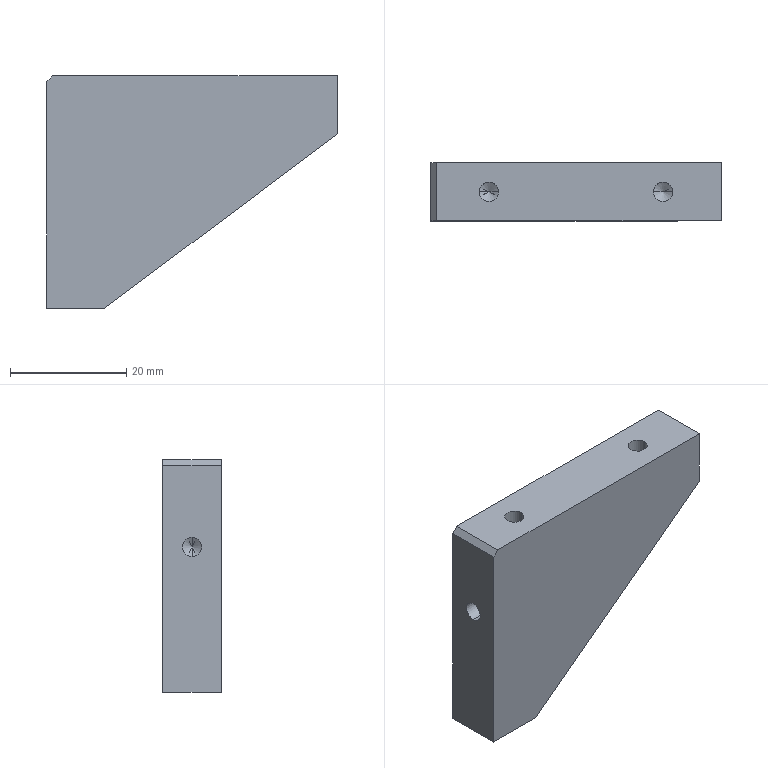Part | STEP file | PN_0035 | 1 solid | 20 faces | box 50 x 10 x 40 mm | volume 13691 mm3 | plane 8 | cylinder 6 | cone 6 | commonest cylinder face diameters 3.3 x6
STEP:
#1=CARTESIAN_POINT('',(0.,0.,0.));
#2=DIRECTION('',(0.,0.,1.));
#3=DIRECTION('',(1.,0.,0.));
#4=AXIS2_PLACEMENT_3D('',#1,#2,#3);
#5=CARTESIAN_POINT('',(16.65,5.,8.5));
#6=VERTEX_POINT('',#5);
#7=CARTESIAN_POINT('',(16.65,5.,20.));
#8=VERTEX_POINT('',#7);
#9=CARTESIAN_POINT('',(16.65,5.,20.));
#10=DIRECTION('',(0.,0.,1.));
#11=VECTOR('',#10,1.);
#12=LINE('',#9,#11);
#13=CARTESIAN_POINT('',(15.,5.,20.));
#14=DIRECTION('',(0.,0.,1.));
#15=DIRECTION('',(1.,0.,0.));
#16=AXIS2_PLACEMENT_3D('',#13,#14,#15);
#17=CYLINDRICAL_SURFACE('',#16,1.65);
#18=CARTESIAN_POINT('',(6.283,0.));
#19=DIRECTION('',(0.,1.));
#20=VECTOR('',#19,1.);
#21=LINE('',#18,#20);
#22=(GEOMETRIC_REPRESENTATION_CONTEXT(2)PARAMETRIC_REPRESENTATION_CONTEXT()REPRESENTATION_CONTEXT('',''));
#23=DEFINITIONAL_REPRESENTATION('',(#21),#22);
#24=PCURVE('',#17,#23);
#25=CARTESIAN_POINT('',(15.,5.,20.));
#26=DIRECTION('',(0.,0.,1.));
#27=DIRECTION('',(1.,0.,0.));
#28=AXIS2_PLACEMENT_3D('',#25,#26,#27);
#29=CYLINDRICAL_SURFACE('',#28,1.65);
#30=CARTESIAN_POINT('',(0.,0.));
#31=DIRECTION('',(0.,1.));
#32=VECTOR('',#31,1.);
#33=LINE('',#30,#32);
#34=(GEOMETRIC_REPRESENTATION_CONTEXT(2)PARAMETRIC_REPRESENTATION_CONTEXT()REPRESENTATION_CONTEXT('',''));
#35=DEFINITIONAL_REPRESENTATION('',(#33),#34);
#36=PCURVE('',#29,#35);
#37=SURFACE_CURVE('',#12,(#24,#36),.PCURVE_S1.);
#38=EDGE_CURVE('',#6,#8,#37,.T.);
#39=ORIENTED_EDGE('',*,*,#38,.T.);
#40=CARTESIAN_POINT('',(13.35,5.,20.));
#41=VERTEX_POINT('',#40);
#42=CARTESIAN_POINT('',(15.,5.,20.));
#43=DIRECTION('',(0.,0.,1.));
#44=DIRECTION('',(1.,0.,0.));
#45=AXIS2_PLACEMENT_3D('',#42,#43,#44);
#46=CIRCLE('',#45,1.65);
#47=CARTESIAN_POINT('',(0.,0.));
#48=DIRECTION('',(1.,0.));
#49=VECTOR('',#48,1.);
#50=LINE('',#47,#49);
#51=(GEOMETRIC_REPRESENTATION_CONTEXT(2)PARAMETRIC_REPRESENTATION_CONTEXT()REPRESENTATION_CONTEXT('',''));
#52=DEFINITIONAL_REPRESENTATION('',(#50),#51);
#53=PCURVE('',#17,#52);
#54=CARTESIAN_POINT('',(-25.,10.,20.));
#55=DIRECTION('',(0.,0.,-1.));
#56=DIRECTION('',(-1.,0.,0.));
#57=AXIS2_PLACEMENT_3D('',#54,#55,#56);
#58=PLANE('',#57);
#59=CARTESIAN_POINT('',(-41.65,-5.));
#60=CARTESIAN_POINT('',(-41.65,-2.142));
#61=CARTESIAN_POINT('',(-39.175,-3.571));
#62=CARTESIAN_POINT('',(-36.7,-5.));
#63=CARTESIAN_POINT('',(-39.175,-6.429));
#64=CARTESIAN_POINT('',(-41.65,-7.858));
#65=CARTESIAN_POINT('',(-41.65,-5.));
#66=(BOUNDED_CURVE()B_SPLINE_CURVE(2,(#59,#60,#61,#62,#63,#64,#65),.UNSPECIFIED.,.T.,.F.)B_SPLINE_CURVE_WITH_KNOTS((1,2,2,2,2,1),(-2.094,0.,2.094,4.189,6.283,8.378),.UNSPECIFIED.)CURVE()GEOMETRIC_REPRESENTATION_ITEM()RATIONAL_B_SPLINE_CURVE((1.,0.5,1.,0.5,1.,0.5,1.))REPRESENTATION_ITEM(''));
#67=(GEOMETRIC_REPRESENTATION_CONTEXT(2)PARAMETRIC_REPRESENTATION_CONTEXT()REPRESENTATION_CONTEXT('',''));
#68=DEFINITIONAL_REPRESENTATION('',(#66),#67);
#69=PCURVE('',#58,#68);
#70=SURFACE_CURVE('',#46,(#53,#69),.PCURVE_S1.);
#71=EDGE_CURVE('',#41,#8,#70,.T.);
#72=ORIENTED_EDGE('',*,*,#71,.F.);
#73=CARTESIAN_POINT('',(13.35,5.,8.5));
#74=VERTEX_POINT('',#73);
#75=CARTESIAN_POINT('',(13.35,5.,20.));
#76=DIRECTION('',(0.,0.,1.));
#77=VECTOR('',#76,1.);
#78=LINE('',#75,#77);
#79=CARTESIAN_POINT('',(3.142,0.));
#80=DIRECTION('',(0.,1.));
#81=VECTOR('',#80,1.);
#82=LINE('',#79,#81);
#83=(GEOMETRIC_REPRESENTATION_CONTEXT(2)PARAMETRIC_REPRESENTATION_CONTEXT()REPRESENTATION_CONTEXT('',''));
#84=DEFINITIONAL_REPRESENTATION('',(#82),#83);
#85=PCURVE('',#17,#84);
#86=CARTESIAN_POINT('',(3.142,0.));
#87=DIRECTION('',(0.,1.));
#88=VECTOR('',#87,1.);
#89=LINE('',#86,#88);
#90=(GEOMETRIC_REPRESENTATION_CONTEXT(2)PARAMETRIC_REPRESENTATION_CONTEXT()REPRESENTATION_CONTEXT('',''));
#91=DEFINITIONAL_REPRESENTATION('',(#89),#90);
#92=PCURVE('',#29,#91);
#93=SURFACE_CURVE('',#78,(#85,#92),.PCURVE_S1.);
#94=EDGE_CURVE('',#74,#41,#93,.T.);
#95=ORIENTED_EDGE('',*,*,#94,.F.);
#96=CARTESIAN_POINT('',(15.,5.,8.5));
#97=DIRECTION('',(0.,0.,1.));
#98=DIRECTION('',(1.,0.,0.));
#99=AXIS2_PLACEMENT_3D('',#96,#97,#98);
#100=CIRCLE('',#99,1.65);
#101=CARTESIAN_POINT('',(0.,-11.5));
#102=DIRECTION('',(1.,0.));
#103=VECTOR('',#102,1.);
#104=LINE('',#101,#103);
#105=(GEOMETRIC_REPRESENTATION_CONTEXT(2)PARAMETRIC_REPRESENTATION_CONTEXT()REPRESENTATION_CONTEXT('',''));
#106=DEFINITIONAL_REPRESENTATION('',(#104),#105);
#107=PCURVE('',#17,#106);
#108=CARTESIAN_POINT('',(15.,5.,8.5));
#109=DIRECTION('',(0.,0.,1.));
#110=DIRECTION('',(1.,0.,0.));
#111=AXIS2_PLACEMENT_3D('',#108,#109,#110);
#112=CONICAL_SURFACE('',#111,1.65,1.03);
#113=CARTESIAN_POINT('',(0.,0.));
#114=DIRECTION('',(1.,0.));
#115=VECTOR('',#114,1.);
#116=LINE('',#113,#115);
#117=(GEOMETRIC_REPRESENTATION_CONTEXT(2)PARAMETRIC_REPRESENTATION_CONTEXT()REPRESENTATION_CONTEXT('',''));
#118=DEFINITIONAL_REPRESENTATION('',(#116),#117);
#119=PCURVE('',#112,#118);
#120=SURFACE_CURVE('',#100,(#107,#119),.PCURVE_S1.);
#121=EDGE_CURVE('',#74,#6,#120,.T.);
#122=ORIENTED_EDGE('',*,*,#121,.T.);
#123=EDGE_LOOP('',(#39,#72,#95,#122));
#124=FACE_BOUND('',#123,.F.);
#125=ADVANCED_FACE('',(#124),#17,.F.);
#126=ORIENTED_EDGE('',*,*,#121,.F.);
#127=CARTESIAN_POINT('',(15.,5.,7.509));
#128=VERTEX_POINT('',#127);
#129=CARTESIAN_POINT('',(13.35,5.,8.5));
#130=DIRECTION('',(-0.8572,0.,0.515));
#131=VECTOR('',#130,1.);
#132=LINE('',#129,#131);
#133=CARTESIAN_POINT('',(3.142,0.));
#134=DIRECTION('',(0.,1.));
#135=VECTOR('',#134,1.);
#136=LINE('',#133,#135);
#137=(GEOMETRIC_REPRESENTATION_CONTEXT(2)PARAMETRIC_REPRESENTATION_CONTEXT()REPRESENTATION_CONTEXT('',''));
#138=DEFINITIONAL_REPRESENTATION('',(#136),#137);
#139=PCURVE('',#112,#138);
#140=CARTESIAN_POINT('',(15.,5.,8.5));
#141=DIRECTION('',(0.,0.,1.));
#142=DIRECTION('',(1.,0.,0.));
#143=AXIS2_PLACEMENT_3D('',#140,#141,#142);
#144=CONICAL_SURFACE('',#143,1.65,1.03);
#145=CARTESIAN_POINT('',(3.142,0.));
#146=DIRECTION('',(0.,1.));
#147=VECTOR('',#146,1.);
#148=LINE('',#145,#147);
#149=(GEOMETRIC_REPRESENTATION_CONTEXT(2)PARAMETRIC_REPRESENTATION_CONTEXT()REPRESENTATION_CONTEXT('',''));
#150=DEFINITIONAL_REPRESENTATION('',(#148),#149);
#151=PCURVE('',#144,#150);
#152=SURFACE_CURVE('',#132,(#139,#151),.PCURVE_S1.);
#153=EDGE_CURVE('',#128,#74,#152,.T.);
#154=ORIENTED_EDGE('',*,*,#153,.F.);
#155=CARTESIAN_POINT('',(16.65,5.,8.5));
#156=DIRECTION('',(0.8572,0.,0.515));
#157=VECTOR('',#156,1.);
#158=LINE('',#155,#157);
#159=CARTESIAN_POINT('',(6.283,0.));
#160=DIRECTION('',(0.,1.));
#161=VECTOR('',#160,1.);
#162=LINE('',#159,#161);
#163=(GEOMETRIC_REPRESENTATION_CONTEXT(2)PARAMETRIC_REPRESENTATION_CONTEXT()REPRESENTATION_CONTEXT('',''));
#164=DEFINITIONAL_REPRESENTATION('',(#162),#163);
#165=PCURVE('',#112,#164);
#166=CARTESIAN_POINT('',(0.,0.));
#167=DIRECTION('',(0.,1.));
#168=VECTOR('',#167,1.);
#169=LINE('',#166,#168);
#170=(GEOMETRIC_REPRESENTATION_CONTEXT(2)PARAMETRIC_REPRESENTATION_CONTEXT()REPRESENTATION_CONTEXT('',''));
#171=DEFINITIONAL_REPRESENTATION('',(#169),#170);
#172=PCURVE('',#144,#171);
#173=SURFACE_CURVE('',#158,(#165,#172),.PCURVE_S1.);
#174=EDGE_CURVE('',#128,#6,#173,.T.);
#175=ORIENTED_EDGE('',*,*,#174,.T.);
#176=EDGE_LOOP('',(#126,#154,#175));
#177=FACE_BOUND('',#176,.F.);
#178=ADVANCED_FACE('',(#177),#112,.F.);
#179=CARTESIAN_POINT('',(-13.35,5.,8.5));
#180=VERTEX_POINT('',#179);
#181=CARTESIAN_POINT('',(-13.35,5.,20.));
#182=VERTEX_POINT('',#181);
#183=CARTESIAN_POINT('',(-13.35,5.,20.));
#184=DIRECTION('',(0.,0.,1.));
#185=VECTOR('',#184,1.);
#186=LINE('',#183,#185);
#187=CARTESIAN_POINT('',(-15.,5.,20.));
#188=DIRECTION('',(0.,0.,1.));
#189=DIRECTION('',(1.,0.,0.));
#190=AXIS2_PLACEMENT_3D('',#187,#188,#189);
#191=CYLINDRICAL_SURFACE('',#190,1.65);
#192=CARTESIAN_POINT('',(6.283,0.));
#193=DIRECTION('',(0.,1.));
#194=VECTOR('',#193,1.);
#195=LINE('',#192,#194);
#196=(GEOMETRIC_REPRESENTATION_CONTEXT(2)PARAMETRIC_REPRESENTATION_CONTEXT()REPRESENTATION_CONTEXT('',''));
#197=DEFINITIONAL_REPRESENTATION('',(#195),#196);
#198=PCURVE('',#191,#197);
#199=CARTESIAN_POINT('',(-15.,5.,20.));
#200=DIRECTION('',(0.,0.,1.));
#201=DIRECTION('',(1.,0.,0.));
#202=AXIS2_PLACEMENT_3D('',#199,#200,#201);
#203=CYLINDRICAL_SURFACE('',#202,1.65);
#204=CARTESIAN_POINT('',(0.,0.));
#205=DIRECTION('',(0.,1.));
#206=VECTOR('',#205,1.);
#207=LINE('',#204,#206);
#208=(GEOMETRIC_REPRESENTATION_CONTEXT(2)PARAMETRIC_REPRESENTATION_CONTEXT()REPRESENTATION_CONTEXT('',''));
#209=DEFINITIONAL_REPRESENTATION('',(#207),#208);
#210=PCURVE('',#203,#209);
#211=SURFACE_CURVE('',#186,(#198,#210),.PCURVE_S1.);
#212=EDGE_CURVE('',#180,#182,#211,.T.);
#213=ORIENTED_EDGE('',*,*,#212,.T.);
#214=CARTESIAN_POINT('',(-16.65,5.,20.));
#215=VERTEX_POINT('',#214);
#216=CARTESIAN_POINT('',(-15.,5.,20.));
#217=DIRECTION('',(0.,0.,1.));
#218=DIRECTION('',(1.,0.,0.));
#219=AXIS2_PLACEMENT_3D('',#216,#217,#218);
#220=CIRCLE('',#219,1.65);
#221=CARTESIAN_POINT('',(0.,0.));
#222=DIRECTION('',(1.,0.));
#223=VECTOR('',#222,1.);
#224=LINE('',#221,#223);
#225=(GEOMETRIC_REPRESENTATION_CONTEXT(2)PARAMETRIC_REPRESENTATION_CONTEXT()REPRESENTATION_CONTEXT('',''));
#226=DEFINITIONAL_REPRESENTATION('',(#224),#225);
#227=PCURVE('',#191,#226);
#228=CARTESIAN_POINT('',(-11.65,-5.));
#229=CARTESIAN_POINT('',(-11.65,-2.142));
#230=CARTESIAN_POINT('',(-9.175,-3.571));
#231=CARTESIAN_POINT('',(-6.7,-5.));
#232=CARTESIAN_POINT('',(-9.175,-6.429));
#233=CARTESIAN_POINT('',(-11.65,-7.858));
#234=CARTESIAN_POINT('',(-11.65,-5.));
#235=(BOUNDED_CURVE()B_SPLINE_CURVE(2,(#228,#229,#230,#231,#232,#233,#234),.UNSPECIFIED.,.T.,.F.)B_SPLINE_CURVE_WITH_KNOTS((1,2,2,2,2,1),(-2.094,0.,2.094,4.189,6.283,8.378),.UNSPECIFIED.)CURVE()GEOMETRIC_REPRESENTATION_ITEM()RATIONAL_B_SPLINE_CURVE((1.,0.5,1.,0.5,1.,0.5,1.))REPRESENTATION_ITEM(''));
#236=(GEOMETRIC_REPRESENTATION_CONTEXT(2)PARAMETRIC_REPRESENTATION_CONTEXT()REPRESENTATION_CONTEXT('',''));
#237=DEFINITIONAL_REPRESENTATION('',(#235),#236);
#238=PCURVE('',#58,#237);
#239=SURFACE_CURVE('',#220,(#227,#238),.PCURVE_S1.);
#240=EDGE_CURVE('',#215,#182,#239,.T.);
#241=ORIENTED_EDGE('',*,*,#240,.F.);
#242=CARTESIAN_POINT('',(-16.65,5.,8.5));
#243=VERTEX_POINT('',#242);
#244=CARTESIAN_POINT('',(-16.65,5.,20.));
#245=DIRECTION('',(0.,0.,1.));
#246=VECTOR('',#245,1.);
#247=LINE('',#244,#246);
#248=CARTESIAN_POINT('',(3.142,0.));
#249=DIRECTION('',(0.,1.));
#250=VECTOR('',#249,1.);
#251=LINE('',#248,#250);
#252=(GEOMETRIC_REPRESENTATION_CONTEXT(2)PARAMETRIC_REPRESENTATION_CONTEXT()REPRESENTATION_CONTEXT('',''));
#253=DEFINITIONAL_REPRESENTATION('',(#251),#252);
#254=PCURVE('',#191,#253);
#255=CARTESIAN_POINT('',(3.142,0.));
#256=DIRECTION('',(0.,1.));
#257=VECTOR('',#256,1.);
#258=LINE('',#255,#257);
#259=(GEOMETRIC_REPRESENTATION_CONTEXT(2)PARAMETRIC_REPRESENTATION_CONTEXT()REPRESENTATION_CONTEXT('',''));
#260=DEFINITIONAL_REPRESENTATION('',(#258),#259);
#261=PCURVE('',#203,#260);
#262=SURFACE_CURVE('',#247,(#254,#261),.PCURVE_S1.);
#263=EDGE_CURVE('',#243,#215,#262,.T.);
#264=ORIENTED_EDGE('',*,*,#263,.F.);
#265=CARTESIAN_POINT('',(-15.,5.,8.5));
#266=DIRECTION('',(0.,0.,1.));
#267=DIRECTION('',(1.,0.,0.));
#268=AXIS2_PLACEMENT_3D('',#265,#266,#267);
#269=CIRCLE('',#268,1.65);
#270=CARTESIAN_POINT('',(0.,-11.5));
#271=DIRECTION('',(1.,0.));
#272=VECTOR('',#271,1.);
#273=LINE('',#270,#272);
#274=(GEOMETRIC_REPRESENTATION_CONTEXT(2)PARAMETRIC_REPRESENTATION_CONTEXT()REPRESENTATION_CONTEXT('',''));
#275=DEFINITIONAL_REPRESENTATION('',(#273),#274);
#276=PCURVE('',#191,#275);
#277=CARTESIAN_POINT('',(-15.,5.,8.5));
#278=DIRECTION('',(0.,0.,1.));
#279=DIRECTION('',(1.,0.,0.));
#280=AXIS2_PLACEMENT_3D('',#277,#278,#279);
#281=CONICAL_SURFACE('',#280,1.65,1.03);
#282=CARTESIAN_POINT('',(0.,0.));
#283=DIRECTION('',(1.,0.));
#284=VECTOR('',#283,1.);
#285=LINE('',#282,#284);
#286=(GEOMETRIC_REPRESENTATION_CONTEXT(2)PARAMETRIC_REPRESENTATION_CONTEXT()REPRESENTATION_CONTEXT('',''));
#287=DEFINITIONAL_REPRESENTATION('',(#285),#286);
#288=PCURVE('',#281,#287);
#289=SURFACE_CURVE('',#269,(#276,#288),.PCURVE_S1.);
#290=EDGE_CURVE('',#243,#180,#289,.T.);
#291=ORIENTED_EDGE('',*,*,#290,.T.);
#292=EDGE_LOOP('',(#213,#241,#264,#291));
#293=FACE_BOUND('',#292,.F.);
#294=ADVANCED_FACE('',(#293),#191,.F.);
#295=ORIENTED_EDGE('',*,*,#290,.F.);
#296=CARTESIAN_POINT('',(-15.,5.,7.509));
#297=VERTEX_POINT('',#296);
#298=CARTESIAN_POINT('',(-16.65,5.,8.5));
#299=DIRECTION('',(-0.8572,0.,0.515));
#300=VECTOR('',#299,1.);
#301=LINE('',#298,#300);
#302=CARTESIAN_POINT('',(3.142,0.));
#303=DIRECTION('',(0.,1.));
#304=VECTOR('',#303,1.);
#305=LINE('',#302,#304);
#306=(GEOMETRIC_REPRESENTATION_CONTEXT(2)PARAMETRIC_REPRESENTATION_CONTEXT()REPRESENTATION_CONTEXT('',''));
#307=DEFINITIONAL_REPRESENTATION('',(#305),#306);
#308=PCURVE('',#281,#307);
#309=CARTESIAN_POINT('',(-15.,5.,8.5));
#310=DIRECTION('',(0.,0.,1.));
#311=DIRECTION('',(1.,0.,0.));
#312=AXIS2_PLACEMENT_3D('',#309,#310,#311);
#313=CONICAL_SURFACE('',#312,1.65,1.03);
#314=CARTESIAN_POINT('',(3.142,0.));
#315=DIRECTION('',(0.,1.));
#316=VECTOR('',#315,1.);
#317=LINE('',#314,#316);
#318=(GEOMETRIC_REPRESENTATION_CONTEXT(2)PARAMETRIC_REPRESENTATION_CONTEXT()REPRESENTATION_CONTEXT('',''));
#319=DEFINITIONAL_REPRESENTATION('',(#317),#318);
#320=PCURVE('',#313,#319);
#321=SURFACE_CURVE('',#301,(#308,#320),.PCURVE_S1.);
#322=EDGE_CURVE('',#297,#243,#321,.T.);
#323=ORIENTED_EDGE('',*,*,#322,.F.);
#324=CARTESIAN_POINT('',(-13.35,5.,8.5));
#325=DIRECTION('',(0.8572,0.,0.515));
#326=VECTOR('',#325,1.);
#327=LINE('',#324,#326);
#328=CARTESIAN_POINT('',(6.283,0.));
#329=DIRECTION('',(0.,1.));
#330=VECTOR('',#329,1.);
#331=LINE('',#328,#330);
#332=(GEOMETRIC_REPRESENTATION_CONTEXT(2)PARAMETRIC_REPRESENTATION_CONTEXT()REPRESENTATION_CONTEXT('',''));
#333=DEFINITIONAL_REPRESENTATION('',(#331),#332);
#334=PCURVE('',#281,#333);
#335=CARTESIAN_POINT('',(0.,0.));
#336=DIRECTION('',(0.,1.));
#337=VECTOR('',#336,1.);
#338=LINE('',#335,#337);
#339=(GEOMETRIC_REPRESENTATION_CONTEXT(2)PARAMETRIC_REPRESENTATION_CONTEXT()REPRESENTATION_CONTEXT('',''));
#340=DEFINITIONAL_REPRESENTATION('',(#338),#339);
#341=PCURVE('',#313,#340);
#342=SURFACE_CURVE('',#327,(#334,#341),.PCURVE_S1.);
#343=EDGE_CURVE('',#297,#180,#342,.T.);
#344=ORIENTED_EDGE('',*,*,#343,.T.);
#345=EDGE_LOOP('',(#295,#323,#344));
#346=FACE_BOUND('',#345,.F.);
#347=ADVANCED_FACE('',(#346),#281,.F.);
#348=CARTESIAN_POINT('',(-13.5,5.,6.65));
#349=VERTEX_POINT('',#348);
#350=CARTESIAN_POINT('',(-25.,5.,6.65));
#351=VERTEX_POINT('',#350);
#352=CARTESIAN_POINT('',(-25.,5.,6.65));
#353=DIRECTION('',(-1.,0.,0.));
#354=VECTOR('',#353,1.);
#355=LINE('',#352,#354);
#356=CARTESIAN_POINT('',(-25.,5.,5.));
#357=DIRECTION('',(-1.,0.,0.));
#358=DIRECTION('',(0.,0.,1.));
#359=AXIS2_PLACEMENT_3D('',#356,#357,#358);
#360=CYLINDRICAL_SURFACE('',#359,1.65);
#361=CARTESIAN_POINT('',(6.283,0.));
#362=DIRECTION('',(0.,1.));
#363=VECTOR('',#362,1.);
#364=LINE('',#361,#363);
#365=(GEOMETRIC_REPRESENTATION_CONTEXT(2)PARAMETRIC_REPRESENTATION_CONTEXT()REPRESENTATION_CONTEXT('',''));
#366=DEFINITIONAL_REPRESENTATION('',(#364),#365);
#367=PCURVE('',#360,#366);
#368=CARTESIAN_POINT('',(-25.,5.,5.));
#369=DIRECTION('',(-1.,0.,0.));
#370=DIRECTION('',(0.,0.,1.));
#371=AXIS2_PLACEMENT_3D('',#368,#369,#370);
#372=CYLINDRICAL_SURFACE('',#371,1.65);
#373=CARTESIAN_POINT('',(0.,0.));
#374=DIRECTION('',(0.,1.));
#375=VECTOR('',#374,1.);
#376=LINE('',#373,#375);
#377=(GEOMETRIC_REPRESENTATION_CONTEXT(2)PARAMETRIC_REPRESENTATION_CONTEXT()REPRESENTATION_CONTEXT('',''));
#378=DEFINITIONAL_REPRESENTATION('',(#376),#377);
#379=PCURVE('',#372,#378);
#380=SURFACE_CURVE('',#355,(#367,#379),.PCURVE_S1.);
#381=EDGE_CURVE('',#349,#351,#380,.T.);
#382=ORIENTED_EDGE('',*,*,#381,.T.);
#383=CARTESIAN_POINT('',(-25.,5.,3.35));
#384=VERTEX_POINT('',#383);
#385=CARTESIAN_POINT('',(-25.,5.,5.));
#386=DIRECTION('',(-1.,0.,0.));
#387=DIRECTION('',(0.,0.,1.));
#388=AXIS2_PLACEMENT_3D('',#385,#386,#387);
#389=CIRCLE('',#388,1.65);
#390=CARTESIAN_POINT('',(0.,0.));
#391=DIRECTION('',(1.,0.));
#392=VECTOR('',#391,1.);
#393=LINE('',#390,#392);
#394=(GEOMETRIC_REPRESENTATION_CONTEXT(2)PARAMETRIC_REPRESENTATION_CONTEXT()REPRESENTATION_CONTEXT('',''));
#395=DEFINITIONAL_REPRESENTATION('',(#393),#394);
#396=PCURVE('',#360,#395);
#397=CARTESIAN_POINT('',(-25.,10.,20.));
#398=DIRECTION('',(1.,0.,0.));
#399=DIRECTION('',(0.,0.,-1.));
#400=AXIS2_PLACEMENT_3D('',#397,#398,#399);
#401=PLANE('',#400);
#402=CARTESIAN_POINT('',(13.35,-5.));
#403=CARTESIAN_POINT('',(13.35,-2.142));
#404=CARTESIAN_POINT('',(15.825,-3.571));
#405=CARTESIAN_POINT('',(18.3,-5.));
#406=CARTESIAN_POINT('',(15.825,-6.429));
#407=CARTESIAN_POINT('',(13.35,-7.858));
#408=CARTESIAN_POINT('',(13.35,-5.));
#409=(BOUNDED_CURVE()B_SPLINE_CURVE(2,(#402,#403,#404,#405,#406,#407,#408),.UNSPECIFIED.,.T.,.F.)B_SPLINE_CURVE_WITH_KNOTS((1,2,2,2,2,1),(-2.094,0.,2.094,4.189,6.283,8.378),.UNSPECIFIED.)CURVE()GEOMETRIC_REPRESENTATION_ITEM()RATIONAL_B_SPLINE_CURVE((1.,0.5,1.,0.5,1.,0.5,1.))REPRESENTATION_ITEM(''));
#410=(GEOMETRIC_REPRESENTATION_CONTEXT(2)PARAMETRIC_REPRESENTATION_CONTEXT()REPRESENTATION_CONTEXT('',''));
#411=DEFINITIONAL_REPRESENTATION('',(#409),#410);
#412=PCURVE('',#401,#411);
#413=SURFACE_CURVE('',#389,(#396,#412),.PCURVE_S1.);
#414=EDGE_CURVE('',#384,#351,#413,.T.);
#415=ORIENTED_EDGE('',*,*,#414,.F.);
#416=CARTESIAN_POINT('',(-13.5,5.,3.35));
#417=VERTEX_POINT('',#416);
#418=CARTESIAN_POINT('',(-25.,5.,3.35));
#419=DIRECTION('',(-1.,0.,0.));
#420=VECTOR('',#419,1.);
#421=LINE('',#418,#420);
#422=CARTESIAN_POINT('',(3.142,0.));
#423=DIRECTION('',(0.,1.));
#424=VECTOR('',#423,1.);
#425=LINE('',#422,#424);
#426=(GEOMETRIC_REPRESENTATION_CONTEXT(2)PARAMETRIC_REPRESENTATION_CONTEXT()REPRESENTATION_CONTEXT('',''));
#427=DEFINITIONAL_REPRESENTATION('',(#425),#426);
#428=PCURVE('',#360,#427);
#429=CARTESIAN_POINT('',(3.142,0.));
#430=DIRECTION('',(0.,1.));
#431=VECTOR('',#430,1.);
#432=LINE('',#429,#431);
#433=(GEOMETRIC_REPRESENTATION_CONTEXT(2)PARAMETRIC_REPRESENTATION_CONTEXT()REPRESENTATION_CONTEXT('',''));
#434=DEFINITIONAL_REPRESENTATION('',(#432),#433);
#435=PCURVE('',#372,#434);
#436=SURFACE_CURVE('',#421,(#428,#435),.PCURVE_S1.);
#437=EDGE_CURVE('',#417,#384,#436,.T.);
#438=ORIENTED_EDGE('',*,*,#437,.F.);
#439=CARTESIAN_POINT('',(-13.5,5.,5.));
#440=DIRECTION('',(-1.,0.,0.));
#441=DIRECTION('',(0.,0.,1.));
#442=AXIS2_PLACEMENT_3D('',#439,#440,#441);
#443=CIRCLE('',#442,1.65);
#444=CARTESIAN_POINT('',(0.,-11.5));
#445=DIRECTION('',(1.,0.));
#446=VECTOR('',#445,1.);
#447=LINE('',#444,#446);
#448=(GEOMETRIC_REPRESENTATION_CONTEXT(2)PARAMETRIC_REPRESENTATION_CONTEXT()REPRESENTATION_CONTEXT('',''));
#449=DEFINITIONAL_REPRESENTATION('',(#447),#448);
#450=PCURVE('',#360,#449);
#451=CARTESIAN_POINT('',(-13.5,5.,5.));
#452=DIRECTION('',(-1.,0.,0.));
#453=DIRECTION('',(0.,0.,1.));
#454=AXIS2_PLACEMENT_3D('',#451,#452,#453);
#455=CONICAL_SURFACE('',#454,1.65,1.03);
#456=CARTESIAN_POINT('',(0.,0.));
#457=DIRECTION('',(1.,0.));
#458=VECTOR('',#457,1.);
#459=LINE('',#456,#458);
#460=(GEOMETRIC_REPRESENTATION_CONTEXT(2)PARAMETRIC_REPRESENTATION_CONTEXT()REPRESENTATION_CONTEXT('',''));
#461=DEFINITIONAL_REPRESENTATION('',(#459),#460);
#462=PCURVE('',#455,#461);
#463=SURFACE_CURVE('',#443,(#450,#462),.PCURVE_S1.);
#464=EDGE_CURVE('',#417,#349,#463,.T.);
#465=ORIENTED_EDGE('',*,*,#464,.T.);
#466=EDGE_LOOP('',(#382,#415,#438,#465));
#467=FACE_BOUND('',#466,.F.);
#468=ADVANCED_FACE('',(#467),#360,.F.);
#469=ORIENTED_EDGE('',*,*,#464,.F.);
#470=CARTESIAN_POINT('',(-12.509,5.,5.));
#471=VERTEX_POINT('',#470);
#472=CARTESIAN_POINT('',(-13.5,5.,3.35));
#473=DIRECTION('',(-0.515,0.,-0.8572));
#474=VECTOR('',#473,1.);
#475=LINE('',#472,#474);
#476=CARTESIAN_POINT('',(3.142,0.));
#477=DIRECTION('',(0.,1.));
#478=VECTOR('',#477,1.);
#479=LINE('',#476,#478);
#480=(GEOMETRIC_REPRESENTATION_CONTEXT(2)PARAMETRIC_REPRESENTATION_CONTEXT()REPRESENTATION_CONTEXT('',''));
#481=DEFINITIONAL_REPRESENTATION('',(#479),#480);
#482=PCURVE('',#455,#481);
#483=CARTESIAN_POINT('',(-13.5,5.,5.));
#484=DIRECTION('',(-1.,0.,0.));
#485=DIRECTION('',(0.,0.,1.));
#486=AXIS2_PLACEMENT_3D('',#483,#484,#485);
#487=CONICAL_SURFACE('',#486,1.65,1.03);
#488=CARTESIAN_POINT('',(3.142,0.));
#489=DIRECTION('',(0.,1.));
#490=VECTOR('',#489,1.);
#491=LINE('',#488,#490);
#492=(GEOMETRIC_REPRESENTATION_CONTEXT(2)PARAMETRIC_REPRESENTATION_CONTEXT()REPRESENTATION_CONTEXT('',''));
#493=DEFINITIONAL_REPRESENTATION('',(#491),#492);
#494=PCURVE('',#487,#493);
#495=SURFACE_CURVE('',#475,(#482,#494),.PCURVE_S1.);
#496=EDGE_CURVE('',#471,#417,#495,.T.);
#497=ORIENTED_EDGE('',*,*,#496,.F.);
#498=CARTESIAN_POINT('',(-13.5,5.,6.65));
#499=DIRECTION('',(-0.515,0.,0.8572));
#500=VECTOR('',#499,1.);
#501=LINE('',#498,#500);
#502=CARTESIAN_POINT('',(6.283,0.));
#503=DIRECTION('',(0.,1.));
#504=VECTOR('',#503,1.);
#505=LINE('',#502,#504);
#506=(GEOMETRIC_REPRESENTATION_CONTEXT(2)PARAMETRIC_REPRESENTATION_CONTEXT()REPRESENTATION_CONTEXT('',''));
#507=DEFINITIONAL_REPRESENTATION('',(#505),#506);
#508=PCURVE('',#455,#507);
#509=CARTESIAN_POINT('',(0.,0.));
#510=DIRECTION('',(0.,1.));
#511=VECTOR('',#510,1.);
#512=LINE('',#509,#511);
#513=(GEOMETRIC_REPRESENTATION_CONTEXT(2)PARAMETRIC_REPRESENTATION_CONTEXT()REPRESENTATION_CONTEXT('',''));
#514=DEFINITIONAL_REPRESENTATION('',(#512),#513);
#515=PCURVE('',#487,#514);
#516=SURFACE_CURVE('',#501,(#508,#515),.PCURVE_S1.);
#517=EDGE_CURVE('',#471,#349,#516,.T.);
#518=ORIENTED_EDGE('',*,*,#517,.T.);
#519=EDGE_LOOP('',(#469,#497,#518));
#520=FACE_BOUND('',#519,.F.);
#521=ADVANCED_FACE('',(#520),#455,.F.);
#522=CARTESIAN_POINT('',(25.,0.,20.));
#523=VERTEX_POINT('',#522);
#524=CARTESIAN_POINT('',(25.,0.,10.));
#525=VERTEX_POINT('',#524);
#526=CARTESIAN_POINT('',(25.,0.,20.));
#527=DIRECTION('',(0.,0.,-1.));
#528=VECTOR('',#527,1.);
#529=LINE('',#526,#528);
#530=CARTESIAN_POINT('',(25.,10.,20.));
#531=DIRECTION('',(-1.,0.,0.));
#532=DIRECTION('',(0.,0.,1.));
#533=AXIS2_PLACEMENT_3D('',#530,#531,#532);
#534=PLANE('',#533);
#535=CARTESIAN_POINT('',(0.,-10.));
#536=DIRECTION('',(-1.,0.));
#537=VECTOR('',#536,1.);
#538=LINE('',#535,#537);
#539=(GEOMETRIC_REPRESENTATION_CONTEXT(2)PARAMETRIC_REPRESENTATION_CONTEXT()REPRESENTATION_CONTEXT('',''));
#540=DEFINITIONAL_REPRESENTATION('',(#538),#539);
#541=PCURVE('',#534,#540);
#542=CARTESIAN_POINT('',(0.,0.,0.));
#543=DIRECTION('',(0.,-1.,0.));
#544=DIRECTION('',(0.,0.,-1.));
#545=AXIS2_PLACEMENT_3D('',#542,#543,#544);
#546=PLANE('',#545);
#547=CARTESIAN_POINT('',(-20.,25.));
#548=DIRECTION('',(1.,0.));
#549=VECTOR('',#548,1.);
#550=LINE('',#547,#549);
#551=(GEOMETRIC_REPRESENTATION_CONTEXT(2)PARAMETRIC_REPRESENTATION_CONTEXT()REPRESENTATION_CONTEXT('',''));
#552=DEFINITIONAL_REPRESENTATION('',(#550),#551);
#553=PCURVE('',#546,#552);
#554=SURFACE_CURVE('',#529,(#541,#553),.PCURVE_S1.);
#555=EDGE_CURVE('',#523,#525,#554,.T.);
#556=ORIENTED_EDGE('',*,*,#555,.T.);
#557=CARTESIAN_POINT('',(25.,10.,10.));
#558=VERTEX_POINT('',#557);
#559=CARTESIAN_POINT('',(25.,10.,10.));
#560=DIRECTION('',(0.,1.,0.));
#561=VECTOR('',#560,1.);
#562=LINE('',#559,#561);
#563=CARTESIAN_POINT('',(-10.,0.));
#564=DIRECTION('',(0.,1.));
#565=VECTOR('',#564,1.);
#566=LINE('',#563,#565);
#567=(GEOMETRIC_REPRESENTATION_CONTEXT(2)PARAMETRIC_REPRESENTATION_CONTEXT()REPRESENTATION_CONTEXT('',''));
#568=DEFINITIONAL_REPRESENTATION('',(#566),#567);
#569=PCURVE('',#534,#568);
#570=CARTESIAN_POINT('',(-15.,10.,-20.));
#571=DIRECTION('',(-0.6,0.,0.8));
#572=DIRECTION('',(0.,-1.,0.));
#573=AXIS2_PLACEMENT_3D('',#570,#571,#572);
#574=PLANE('',#573);
#575=CARTESIAN_POINT('',(0.,50.));
#576=DIRECTION('',(-1.,0.));
#577=VECTOR('',#576,1.);
#578=LINE('',#575,#577);
#579=(GEOMETRIC_REPRESENTATION_CONTEXT(2)PARAMETRIC_REPRESENTATION_CONTEXT()REPRESENTATION_CONTEXT('',''));
#580=DEFINITIONAL_REPRESENTATION('',(#578),#579);
#581=PCURVE('',#574,#580);
#582=SURFACE_CURVE('',#562,(#569,#581),.PCURVE_S1.);
#583=EDGE_CURVE('',#525,#558,#582,.T.);
#584=ORIENTED_EDGE('',*,*,#583,.T.);
#585=CARTESIAN_POINT('',(25.,10.,20.));
#586=VERTEX_POINT('',#585);
#587=CARTESIAN_POINT('',(25.,10.,20.));
#588=DIRECTION('',(0.,0.,-1.));
#589=VECTOR('',#588,1.);
#590=LINE('',#587,#589);
#591=CARTESIAN_POINT('',(0.,0.));
#592=DIRECTION('',(-1.,0.));
#593=VECTOR('',#592,1.);
#594=LINE('',#591,#593);
#595=(GEOMETRIC_REPRESENTATION_CONTEXT(2)PARAMETRIC_REPRESENTATION_CONTEXT()REPRESENTATION_CONTEXT('',''));
#596=DEFINITIONAL_REPRESENTATION('',(#594),#595);
#597=PCURVE('',#534,#596);
#598=CARTESIAN_POINT('',(0.,10.,0.));
#599=DIRECTION('',(0.,-1.,0.));
#600=DIRECTION('',(0.,0.,-1.));
#601=AXIS2_PLACEMENT_3D('',#598,#599,#600);
#602=PLANE('',#601);
#603=CARTESIAN_POINT('',(-20.,25.));
#604=DIRECTION('',(1.,0.));
#605=VECTOR('',#604,1.);
#606=LINE('',#603,#605);
#607=(GEOMETRIC_REPRESENTATION_CONTEXT(2)PARAMETRIC_REPRESENTATION_CONTEXT()REPRESENTATION_CONTEXT('',''));
#608=DEFINITIONAL_REPRESENTATION('',(#606),#607);
#609=PCURVE('',#602,#608);
#610=SURFACE_CURVE('',#590,(#597,#609),.PCURVE_S1.);
#611=EDGE_CURVE('',#586,#558,#610,.T.);
#612=ORIENTED_EDGE('',*,*,#611,.F.);
#613=CARTESIAN_POINT('',(25.,10.,20.));
#614=DIRECTION('',(0.,-1.,0.));
#615=VECTOR('',#614,1.);
#616=LINE('',#613,#615);
#617=CARTESIAN_POINT('',(0.,0.));
#618=DIRECTION('',(0.,-1.));
#619=VECTOR('',#618,1.);
#620=LINE('',#617,#619);
#621=(GEOMETRIC_REPRESENTATION_CONTEXT(2)PARAMETRIC_REPRESENTATION_CONTEXT()REPRESENTATION_CONTEXT('',''));
#622=DEFINITIONAL_REPRESENTATION('',(#620),#621);
#623=PCURVE('',#534,#622);
#624=CARTESIAN_POINT('',(-50.,0.));
#625=DIRECTION('',(0.,-1.));
#626=VECTOR('',#625,1.);
#627=LINE('',#624,#626);
#628=(GEOMETRIC_REPRESENTATION_CONTEXT(2)PARAMETRIC_REPRESENTATION_CONTEXT()REPRESENTATION_CONTEXT('',''));
#629=DEFINITIONAL_REPRESENTATION('',(#627),#628);
#630=PCURVE('',#58,#629);
#631=SURFACE_CURVE('',#616,(#623,#630),.PCURVE_S1.);
#632=EDGE_CURVE('',#586,#523,#631,.T.);
#633=ORIENTED_EDGE('',*,*,#632,.T.);
#634=EDGE_LOOP('',(#556,#584,#612,#633));
#635=FACE_BOUND('',#634,.T.);
#636=ADVANCED_FACE('',(#635),#534,.F.);
#637=CARTESIAN_POINT('',(-15.,10.,-20.));
#638=VERTEX_POINT('',#637);
#639=CARTESIAN_POINT('',(-25.,10.,-20.));
#640=VERTEX_POINT('',#639);
#641=CARTESIAN_POINT('',(-25.,10.,-20.));
#642=DIRECTION('',(-1.,0.,0.));
#643=VECTOR('',#642,1.);
#644=LINE('',#641,#643);
#645=CARTESIAN_POINT('',(-25.,10.,-20.));
#646=DIRECTION('',(0.,0.,1.));
#647=DIRECTION('',(1.,0.,0.));
#648=AXIS2_PLACEMENT_3D('',#645,#646,#647);
#649=PLANE('',#648);
#650=CARTESIAN_POINT('',(0.,0.));
#651=DIRECTION('',(-1.,0.));
#652=VECTOR('',#651,1.);
#653=LINE('',#650,#652);
#654=(GEOMETRIC_REPRESENTATION_CONTEXT(2)PARAMETRIC_REPRESENTATION_CONTEXT()REPRESENTATION_CONTEXT('',''));
#655=DEFINITIONAL_REPRESENTATION('',(#653),#654);
#656=PCURVE('',#649,#655);
#657=CARTESIAN_POINT('',(20.,-25.));
#658=DIRECTION('',(0.,-1.));
#659=VECTOR('',#658,1.);
#660=LINE('',#657,#659);
#661=(GEOMETRIC_REPRESENTATION_CONTEXT(2)PARAMETRIC_REPRESENTATION_CONTEXT()REPRESENTATION_CONTEXT('',''));
#662=DEFINITIONAL_REPRESENTATION('',(#660),#661);
#663=PCURVE('',#602,#662);
#664=SURFACE_CURVE('',#644,(#656,#663),.PCURVE_S1.);
#665=EDGE_CURVE('',#638,#640,#664,.T.);
#666=ORIENTED_EDGE('',*,*,#665,.F.);
#667=CARTESIAN_POINT('',(-15.,0.,-20.));
#668=VERTEX_POINT('',#667);
#669=CARTESIAN_POINT('',(-15.,10.,-20.));
#670=DIRECTION('',(0.,-1.,0.));
#671=VECTOR('',#670,1.);
#672=LINE('',#669,#671);
#673=CARTESIAN_POINT('',(10.,0.));
#674=DIRECTION('',(0.,-1.));
#675=VECTOR('',#674,1.);
#676=LINE('',#673,#675);
#677=(GEOMETRIC_REPRESENTATION_CONTEXT(2)PARAMETRIC_REPRESENTATION_CONTEXT()REPRESENTATION_CONTEXT('',''));
#678=DEFINITIONAL_REPRESENTATION('',(#676),#677);
#679=PCURVE('',#649,#678);
#680=CARTESIAN_POINT('',(0.,0.));
#681=DIRECTION('',(1.,0.));
#682=VECTOR('',#681,1.);
#683=LINE('',#680,#682);
#684=(GEOMETRIC_REPRESENTATION_CONTEXT(2)PARAMETRIC_REPRESENTATION_CONTEXT()REPRESENTATION_CONTEXT('',''));
#685=DEFINITIONAL_REPRESENTATION('',(#683),#684);
#686=PCURVE('',#574,#685);
#687=SURFACE_CURVE('',#672,(#679,#686),.PCURVE_S1.);
#688=EDGE_CURVE('',#638,#668,#687,.T.);
#689=ORIENTED_EDGE('',*,*,#688,.T.);
#690=CARTESIAN_POINT('',(-25.,0.,-20.));
#691=VERTEX_POINT('',#690);
#692=CARTESIAN_POINT('',(-25.,0.,-20.));
#693=DIRECTION('',(-1.,0.,0.));
#694=VECTOR('',#693,1.);
#695=LINE('',#692,#694);
#696=CARTESIAN_POINT('',(0.,-10.));
#697=DIRECTION('',(-1.,0.));
#698=VECTOR('',#697,1.);
#699=LINE('',#696,#698);
#700=(GEOMETRIC_REPRESENTATION_CONTEXT(2)PARAMETRIC_REPRESENTATION_CONTEXT()REPRESENTATION_CONTEXT('',''));
#701=DEFINITIONAL_REPRESENTATION('',(#699),#700);
#702=PCURVE('',#649,#701);
#703=CARTESIAN_POINT('',(20.,-25.));
#704=DIRECTION('',(0.,-1.));
#705=VECTOR('',#704,1.);
#706=LINE('',#703,#705);
#707=(GEOMETRIC_REPRESENTATION_CONTEXT(2)PARAMETRIC_REPRESENTATION_CONTEXT()REPRESENTATION_CONTEXT('',''));
#708=DEFINITIONAL_REPRESENTATION('',(#706),#707);
#709=PCURVE('',#546,#708);
#710=SURFACE_CURVE('',#695,(#702,#709),.PCURVE_S1.);
#711=EDGE_CURVE('',#668,#691,#710,.T.);
#712=ORIENTED_EDGE('',*,*,#711,.T.);
#713=CARTESIAN_POINT('',(-25.,10.,-20.));
#714=DIRECTION('',(0.,-1.,0.));
#715=VECTOR('',#714,1.);
#716=LINE('',#713,#715);
#717=CARTESIAN_POINT('',(0.,0.));
#718=DIRECTION('',(0.,-1.));
#719=VECTOR('',#718,1.);
#720=LINE('',#717,#719);
#721=(GEOMETRIC_REPRESENTATION_CONTEXT(2)PARAMETRIC_REPRESENTATION_CONTEXT()REPRESENTATION_CONTEXT('',''));
#722=DEFINITIONAL_REPRESENTATION('',(#720),#721);
#723=PCURVE('',#649,#722);
#724=CARTESIAN_POINT('',(40.,0.));
#725=DIRECTION('',(0.,-1.));
#726=VECTOR('',#725,1.);
#727=LINE('',#724,#726);
#728=(GEOMETRIC_REPRESENTATION_CONTEXT(2)PARAMETRIC_REPRESENTATION_CONTEXT()REPRESENTATION_CONTEXT('',''));
#729=DEFINITIONAL_REPRESENTATION('',(#727),#728);
#730=PCURVE('',#401,#729);
#731=SURFACE_CURVE('',#716,(#723,#730),.PCURVE_S1.);
#732=EDGE_CURVE('',#640,#691,#731,.T.);
#733=ORIENTED_EDGE('',*,*,#732,.F.);
#734=EDGE_LOOP('',(#666,#689,#712,#733));
#735=FACE_BOUND('',#734,.T.);
#736=ADVANCED_FACE('',(#735),#649,.F.);
#737=CARTESIAN_POINT('',(-25.,5.,5.));
#738=DIRECTION('',(-1.,0.,0.));
#739=DIRECTION('',(0.,0.,1.));
#740=AXIS2_PLACEMENT_3D('',#737,#738,#739);
#741=CIRCLE('',#740,1.65);
#742=CARTESIAN_POINT('',(13.35,-5.));
#743=CARTESIAN_POINT('',(13.35,-2.142));
#744=CARTESIAN_POINT('',(15.825,-3.571));
#745=CARTESIAN_POINT('',(18.3,-5.));
#746=CARTESIAN_POINT('',(15.825,-6.429));
#747=CARTESIAN_POINT('',(13.35,-7.858));
#748=CARTESIAN_POINT('',(13.35,-5.));
#749=(BOUNDED_CURVE()B_SPLINE_CURVE(2,(#742,#743,#744,#745,#746,#747,#748),.UNSPECIFIED.,.T.,.F.)B_SPLINE_CURVE_WITH_KNOTS((1,2,2,2,2,1),(-2.094,0.,2.094,4.189,6.283,8.378),.UNSPECIFIED.)CURVE()GEOMETRIC_REPRESENTATION_ITEM()RATIONAL_B_SPLINE_CURVE((1.,0.5,1.,0.5,1.,0.5,1.))REPRESENTATION_ITEM(''));
#750=(GEOMETRIC_REPRESENTATION_CONTEXT(2)PARAMETRIC_REPRESENTATION_CONTEXT()REPRESENTATION_CONTEXT('',''));
#751=DEFINITIONAL_REPRESENTATION('',(#749),#750);
#752=PCURVE('',#401,#751);
#753=CARTESIAN_POINT('',(0.,0.));
#754=DIRECTION('',(1.,0.));
#755=VECTOR('',#754,1.);
#756=LINE('',#753,#755);
#757=(GEOMETRIC_REPRESENTATION_CONTEXT(2)PARAMETRIC_REPRESENTATION_CONTEXT()REPRESENTATION_CONTEXT('',''));
#758=DEFINITIONAL_REPRESENTATION('',(#756),#757);
#759=PCURVE('',#372,#758);
#760=SURFACE_CURVE('',#741,(#752,#759),.PCURVE_S1.);
#761=EDGE_CURVE('',#351,#384,#760,.T.);
#762=ORIENTED_EDGE('',*,*,#761,.F.);
#763=ORIENTED_EDGE('',*,*,#414,.F.);
#764=EDGE_LOOP('',(#762,#763));
#765=FACE_BOUND('',#764,.T.);
#766=CARTESIAN_POINT('',(-25.,0.,19.));
#767=VERTEX_POINT('',#766);
#768=CARTESIAN_POINT('',(-25.,0.,20.));
#769=DIRECTION('',(0.,0.,1.));
#770=VECTOR('',#769,1.);
#771=LINE('',#768,#770);
#772=CARTESIAN_POINT('',(0.,-10.));
#773=DIRECTION('',(-1.,0.));
#774=VECTOR('',#773,1.);
#775=LINE('',#772,#774);
#776=(GEOMETRIC_REPRESENTATION_CONTEXT(2)PARAMETRIC_REPRESENTATION_CONTEXT()REPRESENTATION_CONTEXT('',''));
#777=DEFINITIONAL_REPRESENTATION('',(#775),#776);
#778=PCURVE('',#401,#777);
#779=CARTESIAN_POINT('',(-20.,-25.));
#780=DIRECTION('',(-1.,0.));
#781=VECTOR('',#780,1.);
#782=LINE('',#779,#781);
#783=(GEOMETRIC_REPRESENTATION_CONTEXT(2)PARAMETRIC_REPRESENTATION_CONTEXT()REPRESENTATION_CONTEXT('',''));
#784=DEFINITIONAL_REPRESENTATION('',(#782),#783);
#785=PCURVE('',#546,#784);
#786=SURFACE_CURVE('',#771,(#778,#785),.PCURVE_S1.);
#787=EDGE_CURVE('',#691,#767,#786,.T.);
#788=ORIENTED_EDGE('',*,*,#787,.T.);
#789=CARTESIAN_POINT('',(-25.,10.,19.));
#790=VERTEX_POINT('',#789);
#791=CARTESIAN_POINT('',(-25.,10.,19.));
#792=DIRECTION('',(0.,1.,0.));
#793=VECTOR('',#792,1.);
#794=LINE('',#791,#793);
#795=CARTESIAN_POINT('',(1.,0.));
#796=DIRECTION('',(0.,1.));
#797=VECTOR('',#796,1.);
#798=LINE('',#795,#797);
#799=(GEOMETRIC_REPRESENTATION_CONTEXT(2)PARAMETRIC_REPRESENTATION_CONTEXT()REPRESENTATION_CONTEXT('',''));
#800=DEFINITIONAL_REPRESENTATION('',(#798),#799);
#801=PCURVE('',#401,#800);
#802=CARTESIAN_POINT('',(-24.,10.,20.));
#803=DIRECTION('',(0.7071,0.,-0.7071));
#804=DIRECTION('',(0.,-1.,0.));
#805=AXIS2_PLACEMENT_3D('',#802,#803,#804);
#806=PLANE('',#805);
#807=CARTESIAN_POINT('',(0.,1.414));
#808=DIRECTION('',(-1.,0.));
#809=VECTOR('',#808,1.);
#810=LINE('',#807,#809);
#811=(GEOMETRIC_REPRESENTATION_CONTEXT(2)PARAMETRIC_REPRESENTATION_CONTEXT()REPRESENTATION_CONTEXT('',''));
#812=DEFINITIONAL_REPRESENTATION('',(#810),#811);
#813=PCURVE('',#806,#812);
#814=SURFACE_CURVE('',#794,(#801,#813),.PCURVE_S1.);
#815=EDGE_CURVE('',#767,#790,#814,.T.);
#816=ORIENTED_EDGE('',*,*,#815,.T.);
#817=CARTESIAN_POINT('',(-25.,10.,20.));
#818=DIRECTION('',(0.,0.,1.));
#819=VECTOR('',#818,1.);
#820=LINE('',#817,#819);
#821=CARTESIAN_POINT('',(0.,0.));
#822=DIRECTION('',(-1.,0.));
#823=VECTOR('',#822,1.);
#824=LINE('',#821,#823);
#825=(GEOMETRIC_REPRESENTATION_CONTEXT(2)PARAMETRIC_REPRESENTATION_CONTEXT()REPRESENTATION_CONTEXT('',''));
#826=DEFINITIONAL_REPRESENTATION('',(#824),#825);
#827=PCURVE('',#401,#826);
#828=CARTESIAN_POINT('',(-20.,-25.));
#829=DIRECTION('',(-1.,0.));
#830=VECTOR('',#829,1.);
#831=LINE('',#828,#830);
#832=(GEOMETRIC_REPRESENTATION_CONTEXT(2)PARAMETRIC_REPRESENTATION_CONTEXT()REPRESENTATION_CONTEXT('',''));
#833=DEFINITIONAL_REPRESENTATION('',(#831),#832);
#834=PCURVE('',#602,#833);
#835=SURFACE_CURVE('',#820,(#827,#834),.PCURVE_S1.);
#836=EDGE_CURVE('',#640,#790,#835,.T.);
#837=ORIENTED_EDGE('',*,*,#836,.F.);
#838=ORIENTED_EDGE('',*,*,#732,.T.);
#839=EDGE_LOOP('',(#788,#816,#837,#838));
#840=FACE_BOUND('',#839,.T.);
#841=ADVANCED_FACE('',(#765,#840),#401,.F.);
#842=CARTESIAN_POINT('',(15.,5.,20.));
#843=DIRECTION('',(0.,0.,1.));
#844=DIRECTION('',(1.,0.,0.));
#845=AXIS2_PLACEMENT_3D('',#842,#843,#844);
#846=CIRCLE('',#845,1.65);
#847=CARTESIAN_POINT('',(-41.65,-5.));
#848=CARTESIAN_POINT('',(-41.65,-2.142));
#849=CARTESIAN_POINT('',(-39.175,-3.571));
#850=CARTESIAN_POINT('',(-36.7,-5.));
#851=CARTESIAN_POINT('',(-39.175,-6.429));
#852=CARTESIAN_POINT('',(-41.65,-7.858));
#853=CARTESIAN_POINT('',(-41.65,-5.));
#854=(BOUNDED_CURVE()B_SPLINE_CURVE(2,(#847,#848,#849,#850,#851,#852,#853),.UNSPECIFIED.,.T.,.F.)B_SPLINE_CURVE_WITH_KNOTS((1,2,2,2,2,1),(-2.094,0.,2.094,4.189,6.283,8.378),.UNSPECIFIED.)CURVE()GEOMETRIC_REPRESENTATION_ITEM()RATIONAL_B_SPLINE_CURVE((1.,0.5,1.,0.5,1.,0.5,1.))REPRESENTATION_ITEM(''));
#855=(GEOMETRIC_REPRESENTATION_CONTEXT(2)PARAMETRIC_REPRESENTATION_CONTEXT()REPRESENTATION_CONTEXT('',''));
#856=DEFINITIONAL_REPRESENTATION('',(#854),#855);
#857=PCURVE('',#58,#856);
#858=CARTESIAN_POINT('',(0.,0.));
#859=DIRECTION('',(1.,0.));
#860=VECTOR('',#859,1.);
#861=LINE('',#858,#860);
#862=(GEOMETRIC_REPRESENTATION_CONTEXT(2)PARAMETRIC_REPRESENTATION_CONTEXT()REPRESENTATION_CONTEXT('',''));
#863=DEFINITIONAL_REPRESENTATION('',(#861),#862);
#864=PCURVE('',#29,#863);
#865=SURFACE_CURVE('',#846,(#857,#864),.PCURVE_S1.);
#866=EDGE_CURVE('',#8,#41,#865,.T.);
#867=ORIENTED_EDGE('',*,*,#866,.F.);
#868=ORIENTED_EDGE('',*,*,#71,.F.);
#869=EDGE_LOOP('',(#867,#868));
#870=FACE_BOUND('',#869,.T.);
#871=CARTESIAN_POINT('',(-15.,5.,20.));
#872=DIRECTION('',(0.,0.,1.));
#873=DIRECTION('',(1.,0.,0.));
#874=AXIS2_PLACEMENT_3D('',#871,#872,#873);
#875=CIRCLE('',#874,1.65);
#876=CARTESIAN_POINT('',(-11.65,-5.));
#877=CARTESIAN_POINT('',(-11.65,-2.142));
#878=CARTESIAN_POINT('',(-9.175,-3.571));
#879=CARTESIAN_POINT('',(-6.7,-5.));
#880=CARTESIAN_POINT('',(-9.175,-6.429));
#881=CARTESIAN_POINT('',(-11.65,-7.858));
#882=CARTESIAN_POINT('',(-11.65,-5.));
#883=(BOUNDED_CURVE()B_SPLINE_CURVE(2,(#876,#877,#878,#879,#880,#881,#882),.UNSPECIFIED.,.T.,.F.)B_SPLINE_CURVE_WITH_KNOTS((1,2,2,2,2,1),(-2.094,0.,2.094,4.189,6.283,8.378),.UNSPECIFIED.)CURVE()GEOMETRIC_REPRESENTATION_ITEM()RATIONAL_B_SPLINE_CURVE((1.,0.5,1.,0.5,1.,0.5,1.))REPRESENTATION_ITEM(''));
#884=(GEOMETRIC_REPRESENTATION_CONTEXT(2)PARAMETRIC_REPRESENTATION_CONTEXT()REPRESENTATION_CONTEXT('',''));
#885=DEFINITIONAL_REPRESENTATION('',(#883),#884);
#886=PCURVE('',#58,#885);
#887=CARTESIAN_POINT('',(0.,0.));
#888=DIRECTION('',(1.,0.));
#889=VECTOR('',#888,1.);
#890=LINE('',#887,#889);
#891=(GEOMETRIC_REPRESENTATION_CONTEXT(2)PARAMETRIC_REPRESENTATION_CONTEXT()REPRESENTATION_CONTEXT('',''));
#892=DEFINITIONAL_REPRESENTATION('',(#890),#891);
#893=PCURVE('',#203,#892);
#894=SURFACE_CURVE('',#875,(#886,#893),.PCURVE_S1.);
#895=EDGE_CURVE('',#182,#215,#894,.T.);
#896=ORIENTED_EDGE('',*,*,#895,.F.);
#897=ORIENTED_EDGE('',*,*,#240,.F.);
#898=EDGE_LOOP('',(#896,#897));
#899=FACE_BOUND('',#898,.T.);
#900=CARTESIAN_POINT('',(-24.,10.,20.));
#901=VERTEX_POINT('',#900);
#902=CARTESIAN_POINT('',(-25.,10.,20.));
#903=DIRECTION('',(1.,0.,0.));
#904=VECTOR('',#903,1.);
#905=LINE('',#902,#904);
#906=CARTESIAN_POINT('',(0.,0.));
#907=DIRECTION('',(-1.,0.));
#908=VECTOR('',#907,1.);
#909=LINE('',#906,#908);
#910=(GEOMETRIC_REPRESENTATION_CONTEXT(2)PARAMETRIC_REPRESENTATION_CONTEXT()REPRESENTATION_CONTEXT('',''));
#911=DEFINITIONAL_REPRESENTATION('',(#909),#910);
#912=PCURVE('',#58,#911);
#913=CARTESIAN_POINT('',(-20.,-25.));
#914=DIRECTION('',(0.,1.));
#915=VECTOR('',#914,1.);
#916=LINE('',#913,#915);
#917=(GEOMETRIC_REPRESENTATION_CONTEXT(2)PARAMETRIC_REPRESENTATION_CONTEXT()REPRESENTATION_CONTEXT('',''));
#918=DEFINITIONAL_REPRESENTATION('',(#916),#917);
#919=PCURVE('',#602,#918);
#920=SURFACE_CURVE('',#905,(#912,#919),.PCURVE_S1.);
#921=EDGE_CURVE('',#901,#586,#920,.T.);
#922=ORIENTED_EDGE('',*,*,#921,.F.);
#923=CARTESIAN_POINT('',(-24.,0.,20.));
#924=VERTEX_POINT('',#923);
#925=CARTESIAN_POINT('',(-24.,10.,20.));
#926=DIRECTION('',(0.,-1.,0.));
#927=VECTOR('',#926,1.);
#928=LINE('',#925,#927);
#929=CARTESIAN_POINT('',(-1.,0.));
#930=DIRECTION('',(0.,-1.));
#931=VECTOR('',#930,1.);
#932=LINE('',#929,#931);
#933=(GEOMETRIC_REPRESENTATION_CONTEXT(2)PARAMETRIC_REPRESENTATION_CONTEXT()REPRESENTATION_CONTEXT('',''));
#934=DEFINITIONAL_REPRESENTATION('',(#932),#933);
#935=PCURVE('',#58,#934);
#936=CARTESIAN_POINT('',(0.,0.));
#937=DIRECTION('',(1.,0.));
#938=VECTOR('',#937,1.);
#939=LINE('',#936,#938);
#940=(GEOMETRIC_REPRESENTATION_CONTEXT(2)PARAMETRIC_REPRESENTATION_CONTEXT()REPRESENTATION_CONTEXT('',''));
#941=DEFINITIONAL_REPRESENTATION('',(#939),#940);
#942=PCURVE('',#806,#941);
#943=SURFACE_CURVE('',#928,(#935,#942),.PCURVE_S1.);
#944=EDGE_CURVE('',#901,#924,#943,.T.);
#945=ORIENTED_EDGE('',*,*,#944,.T.);
#946=CARTESIAN_POINT('',(-25.,0.,20.));
#947=DIRECTION('',(1.,0.,0.));
#948=VECTOR('',#947,1.);
#949=LINE('',#946,#948);
#950=CARTESIAN_POINT('',(0.,-10.));
#951=DIRECTION('',(-1.,0.));
#952=VECTOR('',#951,1.);
#953=LINE('',#950,#952);
#954=(GEOMETRIC_REPRESENTATION_CONTEXT(2)PARAMETRIC_REPRESENTATION_CONTEXT()REPRESENTATION_CONTEXT('',''));
#955=DEFINITIONAL_REPRESENTATION('',(#953),#954);
#956=PCURVE('',#58,#955);
#957=CARTESIAN_POINT('',(-20.,-25.));
#958=DIRECTION('',(0.,1.));
#959=VECTOR('',#958,1.);
#960=LINE('',#957,#959);
#961=(GEOMETRIC_REPRESENTATION_CONTEXT(2)PARAMETRIC_REPRESENTATION_CONTEXT()REPRESENTATION_CONTEXT('',''));
#962=DEFINITIONAL_REPRESENTATION('',(#960),#961);
#963=PCURVE('',#546,#962);
#964=SURFACE_CURVE('',#949,(#956,#963),.PCURVE_S1.);
#965=EDGE_CURVE('',#924,#523,#964,.T.);
#966=ORIENTED_EDGE('',*,*,#965,.T.);
#967=ORIENTED_EDGE('',*,*,#632,.F.);
#968=EDGE_LOOP('',(#922,#945,#966,#967));
#969=FACE_BOUND('',#968,.T.);
#970=ADVANCED_FACE('',(#870,#899,#969),#58,.F.);
#971=ORIENTED_EDGE('',*,*,#611,.T.);
#972=CARTESIAN_POINT('',(-15.,10.,-20.));
#973=DIRECTION('',(-0.8,0.,-0.6));
#974=VECTOR('',#973,1.);
#975=LINE('',#972,#974);
#976=CARTESIAN_POINT('',(20.,-15.));
#977=DIRECTION('',(0.6,-0.8));
#978=VECTOR('',#977,1.);
#979=LINE('',#976,#978);
#980=(GEOMETRIC_REPRESENTATION_CONTEXT(2)PARAMETRIC_REPRESENTATION_CONTEXT()REPRESENTATION_CONTEXT('',''));
#981=DEFINITIONAL_REPRESENTATION('',(#979),#980);
#982=PCURVE('',#602,#981);
#983=CARTESIAN_POINT('',(0.,0.));
#984=DIRECTION('',(0.,-1.));
#985=VECTOR('',#984,1.);
#986=LINE('',#983,#985);
#987=(GEOMETRIC_REPRESENTATION_CONTEXT(2)PARAMETRIC_REPRESENTATION_CONTEXT()REPRESENTATION_CONTEXT('',''));
#988=DEFINITIONAL_REPRESENTATION('',(#986),#987);
#989=PCURVE('',#574,#988);
#990=SURFACE_CURVE('',#975,(#982,#989),.PCURVE_S1.);
#991=EDGE_CURVE('',#558,#638,#990,.T.);
#992=ORIENTED_EDGE('',*,*,#991,.T.);
#993=ORIENTED_EDGE('',*,*,#665,.T.);
#994=ORIENTED_EDGE('',*,*,#836,.T.);
#995=CARTESIAN_POINT('',(-24.,10.,20.));
#996=DIRECTION('',(0.7071,0.,0.7071));
#997=VECTOR('',#996,1.);
#998=LINE('',#995,#997);
#999=CARTESIAN_POINT('',(-20.,-24.));
#1000=DIRECTION('',(-0.7071,0.7071));
#1001=VECTOR('',#1000,1.);
#1002=LINE('',#999,#1001);
#1003=(GEOMETRIC_REPRESENTATION_CONTEXT(2)PARAMETRIC_REPRESENTATION_CONTEXT()REPRESENTATION_CONTEXT('',''));
#1004=DEFINITIONAL_REPRESENTATION('',(#1002),#1003);
#1005=PCURVE('',#602,#1004);
#1006=CARTESIAN_POINT('',(0.,0.));
#1007=DIRECTION('',(0.,-1.));
#1008=VECTOR('',#1007,1.);
#1009=LINE('',#1006,#1008);
#1010=(GEOMETRIC_REPRESENTATION_CONTEXT(2)PARAMETRIC_REPRESENTATION_CONTEXT()REPRESENTATION_CONTEXT('',''));
#1011=DEFINITIONAL_REPRESENTATION('',(#1009),#1010);
#1012=PCURVE('',#806,#1011);
#1013=SURFACE_CURVE('',#998,(#1005,#1012),.PCURVE_S1.);
#1014=EDGE_CURVE('',#790,#901,#1013,.T.);
#1015=ORIENTED_EDGE('',*,*,#1014,.T.);
#1016=ORIENTED_EDGE('',*,*,#921,.T.);
#1017=EDGE_LOOP('',(#971,#992,#993,#994,#1015,#1016));
#1018=FACE_BOUND('',#1017,.T.);
#1019=ADVANCED_FACE('',(#1018),#602,.F.);
#1020=ORIENTED_EDGE('',*,*,#711,.F.);
#1021=CARTESIAN_POINT('',(4.2,0.,-5.6));
#1022=DIRECTION('',(0.8,0.,0.6));
#1023=VECTOR('',#1022,1.);
#1024=LINE('',#1021,#1023);
#1025=CARTESIAN_POINT('',(5.6,4.2));
#1026=DIRECTION('',(-0.6,0.8));
#1027=VECTOR('',#1026,1.);
#1028=LINE('',#1025,#1027);
#1029=(GEOMETRIC_REPRESENTATION_CONTEXT(2)PARAMETRIC_REPRESENTATION_CONTEXT()REPRESENTATION_CONTEXT('',''));
#1030=DEFINITIONAL_REPRESENTATION('',(#1028),#1029);
#1031=PCURVE('',#546,#1030);
#1032=CARTESIAN_POINT('',(10.,24.));
#1033=DIRECTION('',(0.,1.));
#1034=VECTOR('',#1033,1.);
#1035=LINE('',#1032,#1034);
#1036=(GEOMETRIC_REPRESENTATION_CONTEXT(2)PARAMETRIC_REPRESENTATION_CONTEXT()REPRESENTATION_CONTEXT('',''));
#1037=DEFINITIONAL_REPRESENTATION('',(#1035),#1036);
#1038=PCURVE('',#574,#1037);
#1039=SURFACE_CURVE('',#1024,(#1031,#1038),.PCURVE_S1.);
#1040=EDGE_CURVE('',#668,#525,#1039,.T.);
#1041=ORIENTED_EDGE('',*,*,#1040,.T.);
#1042=ORIENTED_EDGE('',*,*,#555,.F.);
#1043=ORIENTED_EDGE('',*,*,#965,.F.);
#1044=CARTESIAN_POINT('',(-22.,0.,22.));
#1045=DIRECTION('',(-0.7071,0.,-0.7071));
#1046=VECTOR('',#1045,1.);
#1047=LINE('',#1044,#1046);
#1048=CARTESIAN_POINT('',(-22.,-22.));
#1049=DIRECTION('',(0.7071,-0.7071));
#1050=VECTOR('',#1049,1.);
#1051=LINE('',#1048,#1050);
#1052=(GEOMETRIC_REPRESENTATION_CONTEXT(2)PARAMETRIC_REPRESENTATION_CONTEXT()REPRESENTATION_CONTEXT('',''));
#1053=DEFINITIONAL_REPRESENTATION('',(#1051),#1052);
#1054=PCURVE('',#546,#1053);
#1055=CARTESIAN_POINT('',(10.,-2.828));
#1056=DIRECTION('',(0.,1.));
#1057=VECTOR('',#1056,1.);
#1058=LINE('',#1055,#1057);
#1059=(GEOMETRIC_REPRESENTATION_CONTEXT(2)PARAMETRIC_REPRESENTATION_CONTEXT()REPRESENTATION_CONTEXT('',''));
#1060=DEFINITIONAL_REPRESENTATION('',(#1058),#1059);
#1061=PCURVE('',#806,#1060);
#1062=SURFACE_CURVE('',#1047,(#1054,#1061),.PCURVE_S1.);
#1063=EDGE_CURVE('',#924,#767,#1062,.T.);
#1064=ORIENTED_EDGE('',*,*,#1063,.T.);
#1065=ORIENTED_EDGE('',*,*,#787,.F.);
#1066=EDGE_LOOP('',(#1020,#1041,#1042,#1043,#1064,#1065));
#1067=FACE_BOUND('',#1066,.T.);
#1068=ADVANCED_FACE('',(#1067),#546,.T.);
#1069=ORIENTED_EDGE('',*,*,#1014,.F.);
#1070=ORIENTED_EDGE('',*,*,#815,.F.);
#1071=ORIENTED_EDGE('',*,*,#1063,.F.);
#1072=ORIENTED_EDGE('',*,*,#944,.F.);
#1073=EDGE_LOOP('',(#1069,#1070,#1071,#1072));
#1074=FACE_BOUND('',#1073,.T.);
#1075=ADVANCED_FACE('',(#1074),#806,.F.);
#1076=ORIENTED_EDGE('',*,*,#991,.F.);
#1077=ORIENTED_EDGE('',*,*,#583,.F.);
#1078=ORIENTED_EDGE('',*,*,#1040,.F.);
#1079=ORIENTED_EDGE('',*,*,#688,.F.);
#1080=EDGE_LOOP('',(#1076,#1077,#1078,#1079));
#1081=FACE_BOUND('',#1080,.T.);
#1082=ADVANCED_FACE('',(#1081),#574,.F.);
#1083=CARTESIAN_POINT('',(-13.5,5.,5.));
#1084=DIRECTION('',(-1.,0.,0.));
#1085=DIRECTION('',(0.,0.,1.));
#1086=AXIS2_PLACEMENT_3D('',#1083,#1084,#1085);
#1087=CIRCLE('',#1086,1.65);
#1088=CARTESIAN_POINT('',(0.,0.));
#1089=DIRECTION('',(1.,0.));
#1090=VECTOR('',#1089,1.);
#1091=LINE('',#1088,#1090);
#1092=(GEOMETRIC_REPRESENTATION_CONTEXT(2)PARAMETRIC_REPRESENTATION_CONTEXT()REPRESENTATION_CONTEXT('',''));
#1093=DEFINITIONAL_REPRESENTATION('',(#1091),#1092);
#1094=PCURVE('',#487,#1093);
#1095=CARTESIAN_POINT('',(0.,-11.5));
#1096=DIRECTION('',(1.,0.));
#1097=VECTOR('',#1096,1.);
#1098=LINE('',#1095,#1097);
#1099=(GEOMETRIC_REPRESENTATION_CONTEXT(2)PARAMETRIC_REPRESENTATION_CONTEXT()REPRESENTATION_CONTEXT('',''));
#1100=DEFINITIONAL_REPRESENTATION('',(#1098),#1099);
#1101=PCURVE('',#372,#1100);
#1102=SURFACE_CURVE('',#1087,(#1094,#1101),.PCURVE_S1.);
#1103=EDGE_CURVE('',#349,#417,#1102,.T.);
#1104=ORIENTED_EDGE('',*,*,#1103,.F.);
#1105=ORIENTED_EDGE('',*,*,#517,.F.);
#1106=ORIENTED_EDGE('',*,*,#496,.T.);
#1107=EDGE_LOOP('',(#1104,#1105,#1106));
#1108=FACE_BOUND('',#1107,.F.);
#1109=ADVANCED_FACE('',(#1108),#487,.F.);
#1110=ORIENTED_EDGE('',*,*,#761,.F.);
#1111=ORIENTED_EDGE('',*,*,#381,.F.);
#1112=ORIENTED_EDGE('',*,*,#1103,.T.);
#1113=ORIENTED_EDGE('',*,*,#437,.T.);
#1114=EDGE_LOOP('',(#1110,#1111,#1112,#1113));
#1115=FACE_BOUND('',#1114,.F.);
#1116=ADVANCED_FACE('',(#1115),#372,.F.);
#1117=CARTESIAN_POINT('',(-15.,5.,8.5));
#1118=DIRECTION('',(0.,0.,1.));
#1119=DIRECTION('',(1.,0.,0.));
#1120=AXIS2_PLACEMENT_3D('',#1117,#1118,#1119);
#1121=CIRCLE('',#1120,1.65);
#1122=CARTESIAN_POINT('',(0.,0.));
#1123=DIRECTION('',(1.,0.));
#1124=VECTOR('',#1123,1.);
#1125=LINE('',#1122,#1124);
#1126=(GEOMETRIC_REPRESENTATION_CONTEXT(2)PARAMETRIC_REPRESENTATION_CONTEXT()REPRESENTATION_CONTEXT('',''));
#1127=DEFINITIONAL_REPRESENTATION('',(#1125),#1126);
#1128=PCURVE('',#313,#1127);
#1129=CARTESIAN_POINT('',(0.,-11.5));
#1130=DIRECTION('',(1.,0.));
#1131=VECTOR('',#1130,1.);
#1132=LINE('',#1129,#1131);
#1133=(GEOMETRIC_REPRESENTATION_CONTEXT(2)PARAMETRIC_REPRESENTATION_CONTEXT()REPRESENTATION_CONTEXT('',''));
#1134=DEFINITIONAL_REPRESENTATION('',(#1132),#1133);
#1135=PCURVE('',#203,#1134);
#1136=SURFACE_CURVE('',#1121,(#1128,#1135),.PCURVE_S1.);
#1137=EDGE_CURVE('',#180,#243,#1136,.T.);
#1138=ORIENTED_EDGE('',*,*,#1137,.F.);
#1139=ORIENTED_EDGE('',*,*,#343,.F.);
#1140=ORIENTED_EDGE('',*,*,#322,.T.);
#1141=EDGE_LOOP('',(#1138,#1139,#1140));
#1142=FACE_BOUND('',#1141,.F.);
#1143=ADVANCED_FACE('',(#1142),#313,.F.);
#1144=ORIENTED_EDGE('',*,*,#895,.F.);
#1145=ORIENTED_EDGE('',*,*,#212,.F.);
#1146=ORIENTED_EDGE('',*,*,#1137,.T.);
#1147=ORIENTED_EDGE('',*,*,#263,.T.);
#1148=EDGE_LOOP('',(#1144,#1145,#1146,#1147));
#1149=FACE_BOUND('',#1148,.F.);
#1150=ADVANCED_FACE('',(#1149),#203,.F.);
#1151=CARTESIAN_POINT('',(15.,5.,8.5));
#1152=DIRECTION('',(0.,0.,1.));
#1153=DIRECTION('',(1.,0.,0.));
#1154=AXIS2_PLACEMENT_3D('',#1151,#1152,#1153);
#1155=CIRCLE('',#1154,1.65);
#1156=CARTESIAN_POINT('',(0.,0.));
#1157=DIRECTION('',(1.,0.));
#1158=VECTOR('',#1157,1.);
#1159=LINE('',#1156,#1158);
#1160=(GEOMETRIC_REPRESENTATION_CONTEXT(2)PARAMETRIC_REPRESENTATION_CONTEXT()REPRESENTATION_CONTEXT('',''));
#1161=DEFINITIONAL_REPRESENTATION('',(#1159),#1160);
#1162=PCURVE('',#144,#1161);
#1163=CARTESIAN_POINT('',(0.,-11.5));
#1164=DIRECTION('',(1.,0.));
#1165=VECTOR('',#1164,1.);
#1166=LINE('',#1163,#1165);
#1167=(GEOMETRIC_REPRESENTATION_CONTEXT(2)PARAMETRIC_REPRESENTATION_CONTEXT()REPRESENTATION_CONTEXT('',''));
#1168=DEFINITIONAL_REPRESENTATION('',(#1166),#1167);
#1169=PCURVE('',#29,#1168);
#1170=SURFACE_CURVE('',#1155,(#1162,#1169),.PCURVE_S1.);
#1171=EDGE_CURVE('',#6,#74,#1170,.T.);
#1172=ORIENTED_EDGE('',*,*,#1171,.F.);
#1173=ORIENTED_EDGE('',*,*,#174,.F.);
#1174=ORIENTED_EDGE('',*,*,#153,.T.);
#1175=EDGE_LOOP('',(#1172,#1173,#1174));
#1176=FACE_BOUND('',#1175,.F.);
#1177=ADVANCED_FACE('',(#1176),#144,.F.);
#1178=ORIENTED_EDGE('',*,*,#866,.F.);
#1179=ORIENTED_EDGE('',*,*,#38,.F.);
#1180=ORIENTED_EDGE('',*,*,#1171,.T.);
#1181=ORIENTED_EDGE('',*,*,#94,.T.);
#1182=EDGE_LOOP('',(#1178,#1179,#1180,#1181));
#1183=FACE_BOUND('',#1182,.F.);
#1184=ADVANCED_FACE('',(#1183),#29,.F.);
#1185=CLOSED_SHELL('',(#125,#178,#294,#347,#468,#521,#636,#736,#841,#970,#1019,#1068,#1075,#1082,#1109,#1116,#1143,#1150,#1177,#1184));
#1186=MANIFOLD_SOLID_BREP('',#1185);
#1187=(LENGTH_UNIT()NAMED_UNIT(*)SI_UNIT(.MILLI.,.METRE.));
#1188=UNCERTAINTY_MEASURE_WITH_UNIT(LENGTH_MEASURE(0.0000001),#1187,'','');
#1189=(NAMED_UNIT(*)PLANE_ANGLE_UNIT()SI_UNIT($,.RADIAN.));
#1190=(NAMED_UNIT(*)SI_UNIT($,.STERADIAN.)SOLID_ANGLE_UNIT());
#1191=(GEOMETRIC_REPRESENTATION_CONTEXT(3)GLOBAL_UNCERTAINTY_ASSIGNED_CONTEXT((#1188))GLOBAL_UNIT_ASSIGNED_CONTEXT((#1187,#1189,#1190))REPRESENTATION_CONTEXT('',''));
#1192=ADVANCED_BREP_SHAPE_REPRESENTATION('',(#4,#1186),#1191);